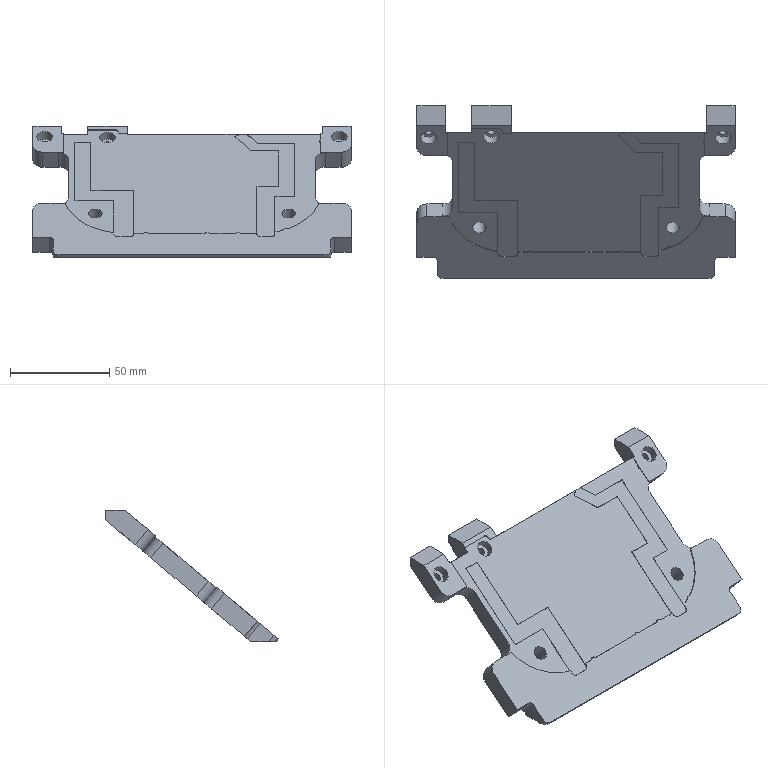Part | SolidWorks | features BaseBody 1 | 1 solid | 130 faces | box 160 x 86.9 x 65.902 mm | volume 123338 mm3 | plane 79 | cylinder 51 | commonest cylinder face diameters 3.3 x11 10 x8 4 x6 4.2 x6 8 x6 6.9 x4